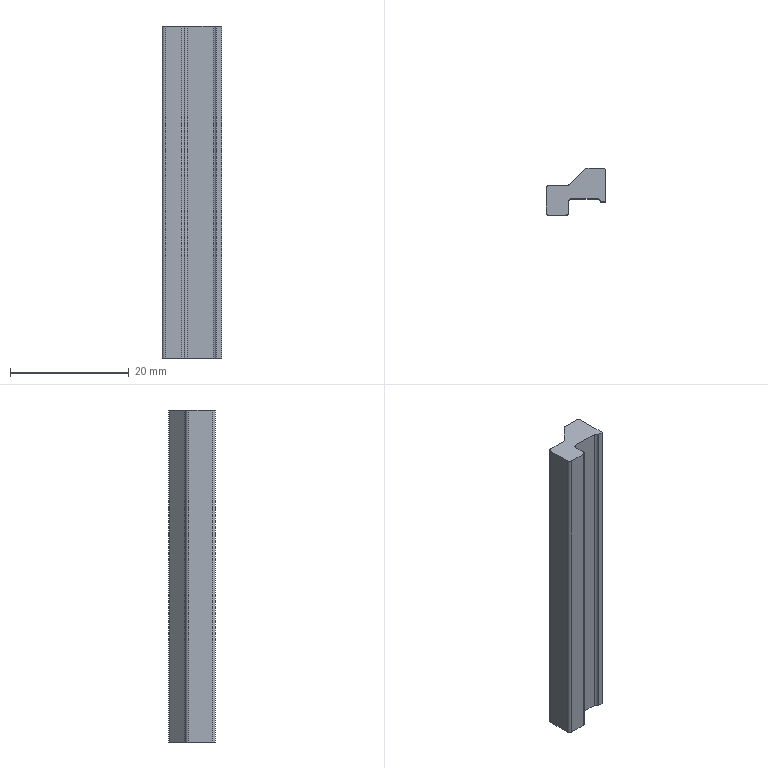Part | NX | features BREP 2 | 2 solids | 40 faces | box 10.056 x 7.899 x 56 mm | volume 5282 mm3 | plane 22 | cylinder 18 | commonest cylinder face diameters 1 x16 188.049 x2
STEP:
#1=CARTESIAN_POINT('',(-0.7746,-1.164,-4.));
#2=VERTEX_POINT('',#1);
#3=CARTESIAN_POINT('',(-0.7746,-1.164,52.));
#4=VERTEX_POINT('',#3);
#5=CARTESIAN_POINT('',(-0.7746,-1.164,0.));
#6=DIRECTION('',(0.,0.,1.));
#7=VECTOR('',#6,1000.);
#8=LINE('',#5,#7);
#9=EDGE_CURVE('',#2,#4,#8,.T.);
#10=ORIENTED_EDGE('',*,*,#9,.T.);
#11=CARTESIAN_POINT('',(-1.275,-1.664,52.));
#12=VERTEX_POINT('',#11);
#13=CARTESIAN_POINT('',(-0.7746,-1.664,52.));
#14=DIRECTION('',(0.,0.,-1.));
#15=DIRECTION('',(1.,0.,0.));
#16=AXIS2_PLACEMENT_3D('',#13,#14,#15);
#17=CIRCLE('',#16,0.5);
#18=EDGE_CURVE('',#12,#4,#17,.T.);
#19=ORIENTED_EDGE('',*,*,#18,.F.);
#20=CARTESIAN_POINT('',(-1.275,-1.664,-4.));
#21=VERTEX_POINT('',#20);
#22=CARTESIAN_POINT('',(-1.275,-1.664,0.));
#23=DIRECTION('',(0.,0.,1.));
#24=VECTOR('',#23,1000.);
#25=LINE('',#22,#24);
#26=EDGE_CURVE('',#21,#12,#25,.T.);
#27=ORIENTED_EDGE('',*,*,#26,.F.);
#28=CARTESIAN_POINT('',(-0.7746,-1.664,-4.));
#29=DIRECTION('',(0.,0.,-1.));
#30=DIRECTION('',(1.,0.,0.));
#31=AXIS2_PLACEMENT_3D('',#28,#29,#30);
#32=CIRCLE('',#31,0.5);
#33=EDGE_CURVE('',#21,#2,#32,.T.);
#34=ORIENTED_EDGE('',*,*,#33,.T.);
#35=EDGE_LOOP('',(#10,#19,#27,#34));
#36=FACE_BOUND('',#35,.T.);
#37=CARTESIAN_POINT('',(-0.7746,-1.664,0.));
#38=DIRECTION('',(0.,0.,1.));
#39=DIRECTION('',(-1.,0.,0.));
#40=AXIS2_PLACEMENT_3D('',#37,#38,#39);
#41=CYLINDRICAL_SURFACE('',#40,0.5);
#42=ADVANCED_FACE('',(#36),#41,.F.);
#43=ORIENTED_EDGE('',*,*,#26,.T.);
#44=CARTESIAN_POINT('',(-1.275,-3.45,52.));
#45=VERTEX_POINT('',#44);
#46=CARTESIAN_POINT('',(-1.275,3.331,52.));
#47=DIRECTION('',(0.,1.,0.));
#48=VECTOR('',#47,1000.);
#49=LINE('',#46,#48);
#50=EDGE_CURVE('',#45,#12,#49,.T.);
#51=ORIENTED_EDGE('',*,*,#50,.F.);
#52=CARTESIAN_POINT('',(-1.275,-3.45,-4.));
#53=VERTEX_POINT('',#52);
#54=CARTESIAN_POINT('',(-1.275,-3.45,0.));
#55=DIRECTION('',(0.,0.,1.));
#56=VECTOR('',#55,1000.);
#57=LINE('',#54,#56);
#58=EDGE_CURVE('',#53,#45,#57,.T.);
#59=ORIENTED_EDGE('',*,*,#58,.F.);
#60=CARTESIAN_POINT('',(-1.275,3.331,-4.));
#61=DIRECTION('',(0.,1.,0.));
#62=VECTOR('',#61,1000.);
#63=LINE('',#60,#62);
#64=EDGE_CURVE('',#53,#21,#63,.T.);
#65=ORIENTED_EDGE('',*,*,#64,.T.);
#66=EDGE_LOOP('',(#43,#51,#59,#65));
#67=FACE_BOUND('',#66,.T.);
#68=CARTESIAN_POINT('',(-1.275,-1.664,0.));
#69=DIRECTION('',(-1.,0.,0.));
#70=DIRECTION('',(0.,1.,0.));
#71=AXIS2_PLACEMENT_3D('',#68,#69,#70);
#72=PLANE('',#71);
#73=ADVANCED_FACE('',(#67),#72,.F.);
#74=ORIENTED_EDGE('',*,*,#58,.T.);
#75=CARTESIAN_POINT('',(-1.775,-3.95,52.));
#76=VERTEX_POINT('',#75);
#77=CARTESIAN_POINT('',(-1.775,-3.45,52.));
#78=DIRECTION('',(0.,0.,1.));
#79=DIRECTION('',(1.,0.,0.));
#80=AXIS2_PLACEMENT_3D('',#77,#78,#79);
#81=CIRCLE('',#80,0.5);
#82=EDGE_CURVE('',#76,#45,#81,.T.);
#83=ORIENTED_EDGE('',*,*,#82,.F.);
#84=CARTESIAN_POINT('',(-1.775,-3.95,-4.));
#85=VERTEX_POINT('',#84);
#86=CARTESIAN_POINT('',(-1.775,-3.95,0.));
#87=DIRECTION('',(0.,0.,1.));
#88=VECTOR('',#87,1000.);
#89=LINE('',#86,#88);
#90=EDGE_CURVE('',#85,#76,#89,.T.);
#91=ORIENTED_EDGE('',*,*,#90,.F.);
#92=CARTESIAN_POINT('',(-1.775,-3.45,-4.));
#93=DIRECTION('',(0.,0.,1.));
#94=DIRECTION('',(1.,0.,0.));
#95=AXIS2_PLACEMENT_3D('',#92,#93,#94);
#96=CIRCLE('',#95,0.5);
#97=EDGE_CURVE('',#85,#53,#96,.T.);
#98=ORIENTED_EDGE('',*,*,#97,.T.);
#99=EDGE_LOOP('',(#74,#83,#91,#98));
#100=FACE_BOUND('',#99,.T.);
#101=CARTESIAN_POINT('',(-1.775,-3.45,0.));
#102=DIRECTION('',(0.,0.,1.));
#103=DIRECTION('',(-1.,0.,0.));
#104=AXIS2_PLACEMENT_3D('',#101,#102,#103);
#105=CYLINDRICAL_SURFACE('',#104,0.5);
#106=ADVANCED_FACE('',(#100),#105,.T.);
#107=ORIENTED_EDGE('',*,*,#90,.T.);
#108=CARTESIAN_POINT('',(-4.531,-3.95,52.));
#109=VERTEX_POINT('',#108);
#110=CARTESIAN_POINT('',(-8.005,-3.95,52.));
#111=DIRECTION('',(1.,0.,0.));
#112=VECTOR('',#111,1000.);
#113=LINE('',#110,#112);
#114=EDGE_CURVE('',#109,#76,#113,.T.);
#115=ORIENTED_EDGE('',*,*,#114,.F.);
#116=CARTESIAN_POINT('',(-4.531,-3.95,-4.));
#117=VERTEX_POINT('',#116);
#118=CARTESIAN_POINT('',(-4.531,-3.95,0.));
#119=DIRECTION('',(0.,0.,1.));
#120=VECTOR('',#119,1000.);
#121=LINE('',#118,#120);
#122=EDGE_CURVE('',#117,#109,#121,.T.);
#123=ORIENTED_EDGE('',*,*,#122,.F.);
#124=CARTESIAN_POINT('',(-8.005,-3.95,-4.));
#125=DIRECTION('',(1.,0.,0.));
#126=VECTOR('',#125,1000.);
#127=LINE('',#124,#126);
#128=EDGE_CURVE('',#117,#85,#127,.T.);
#129=ORIENTED_EDGE('',*,*,#128,.T.);
#130=EDGE_LOOP('',(#107,#115,#123,#129));
#131=FACE_BOUND('',#130,.T.);
#132=CARTESIAN_POINT('',(-1.775,-3.95,0.));
#133=DIRECTION('',(0.,1.,0.));
#134=DIRECTION('',(1.,0.,0.));
#135=AXIS2_PLACEMENT_3D('',#132,#133,#134);
#136=PLANE('',#135);
#137=ADVANCED_FACE('',(#131),#136,.F.);
#138=ORIENTED_EDGE('',*,*,#122,.T.);
#139=CARTESIAN_POINT('',(-5.031,-3.45,52.));
#140=VERTEX_POINT('',#139);
#141=CARTESIAN_POINT('',(-4.531,-3.45,52.));
#142=DIRECTION('',(0.,0.,1.));
#143=DIRECTION('',(1.,0.,0.));
#144=AXIS2_PLACEMENT_3D('',#141,#142,#143);
#145=CIRCLE('',#144,0.5);
#146=EDGE_CURVE('',#140,#109,#145,.T.);
#147=ORIENTED_EDGE('',*,*,#146,.F.);
#148=CARTESIAN_POINT('',(-5.031,-3.45,-4.));
#149=VERTEX_POINT('',#148);
#150=CARTESIAN_POINT('',(-5.031,-3.45,0.));
#151=DIRECTION('',(0.,0.,1.));
#152=VECTOR('',#151,1000.);
#153=LINE('',#150,#152);
#154=EDGE_CURVE('',#149,#140,#153,.T.);
#155=ORIENTED_EDGE('',*,*,#154,.F.);
#156=CARTESIAN_POINT('',(-4.531,-3.45,-4.));
#157=DIRECTION('',(0.,0.,1.));
#158=DIRECTION('',(1.,0.,0.));
#159=AXIS2_PLACEMENT_3D('',#156,#157,#158);
#160=CIRCLE('',#159,0.5);
#161=EDGE_CURVE('',#149,#117,#160,.T.);
#162=ORIENTED_EDGE('',*,*,#161,.T.);
#163=EDGE_LOOP('',(#138,#147,#155,#162));
#164=FACE_BOUND('',#163,.T.);
#165=CARTESIAN_POINT('',(-4.531,-3.45,0.));
#166=DIRECTION('',(0.,0.,1.));
#167=DIRECTION('',(-1.,0.,0.));
#168=AXIS2_PLACEMENT_3D('',#165,#166,#167);
#169=CYLINDRICAL_SURFACE('',#168,0.5);
#170=ADVANCED_FACE('',(#164),#169,.T.);
#171=ORIENTED_EDGE('',*,*,#154,.T.);
#172=CARTESIAN_POINT('',(-5.031,0.5504,52.));
#173=VERTEX_POINT('',#172);
#174=CARTESIAN_POINT('',(-5.031,3.331,52.));
#175=DIRECTION('',(0.,-1.,0.));
#176=VECTOR('',#175,1000.);
#177=LINE('',#174,#176);
#178=EDGE_CURVE('',#173,#140,#177,.T.);
#179=ORIENTED_EDGE('',*,*,#178,.F.);
#180=CARTESIAN_POINT('',(-5.031,0.5504,-4.));
#181=VERTEX_POINT('',#180);
#182=CARTESIAN_POINT('',(-5.031,0.5504,0.));
#183=DIRECTION('',(0.,0.,1.));
#184=VECTOR('',#183,1000.);
#185=LINE('',#182,#184);
#186=EDGE_CURVE('',#181,#173,#185,.T.);
#187=ORIENTED_EDGE('',*,*,#186,.F.);
#188=CARTESIAN_POINT('',(-5.031,3.331,-4.));
#189=DIRECTION('',(0.,-1.,0.));
#190=VECTOR('',#189,1000.);
#191=LINE('',#188,#190);
#192=EDGE_CURVE('',#181,#149,#191,.T.);
#193=ORIENTED_EDGE('',*,*,#192,.T.);
#194=EDGE_LOOP('',(#171,#179,#187,#193));
#195=FACE_BOUND('',#194,.T.);
#196=CARTESIAN_POINT('',(-5.031,-3.45,0.));
#197=DIRECTION('',(1.,0.,0.));
#198=DIRECTION('',(0.,-1.,0.));
#199=AXIS2_PLACEMENT_3D('',#196,#197,#198);
#200=PLANE('',#199);
#201=ADVANCED_FACE('',(#195),#200,.F.);
#202=ORIENTED_EDGE('',*,*,#186,.T.);
#203=CARTESIAN_POINT('',(-4.531,1.05,52.));
#204=VERTEX_POINT('',#203);
#205=CARTESIAN_POINT('',(-4.531,0.5504,52.));
#206=DIRECTION('',(0.,0.,1.));
#207=DIRECTION('',(1.,0.,0.));
#208=AXIS2_PLACEMENT_3D('',#205,#206,#207);
#209=CIRCLE('',#208,0.5);
#210=EDGE_CURVE('',#204,#173,#209,.T.);
#211=ORIENTED_EDGE('',*,*,#210,.F.);
#212=CARTESIAN_POINT('',(-4.531,1.05,-4.));
#213=VERTEX_POINT('',#212);
#214=CARTESIAN_POINT('',(-4.531,1.05,0.));
#215=DIRECTION('',(0.,0.,1.));
#216=VECTOR('',#215,1000.);
#217=LINE('',#214,#216);
#218=EDGE_CURVE('',#213,#204,#217,.T.);
#219=ORIENTED_EDGE('',*,*,#218,.F.);
#220=CARTESIAN_POINT('',(-4.531,0.5504,-4.));
#221=DIRECTION('',(0.,0.,1.));
#222=DIRECTION('',(1.,0.,0.));
#223=AXIS2_PLACEMENT_3D('',#220,#221,#222);
#224=CIRCLE('',#223,0.5);
#225=EDGE_CURVE('',#213,#181,#224,.T.);
#226=ORIENTED_EDGE('',*,*,#225,.T.);
#227=EDGE_LOOP('',(#202,#211,#219,#226));
#228=FACE_BOUND('',#227,.T.);
#229=CARTESIAN_POINT('',(-4.531,0.5504,0.));
#230=DIRECTION('',(0.,0.,1.));
#231=DIRECTION('',(-1.,0.,0.));
#232=AXIS2_PLACEMENT_3D('',#229,#230,#231);
#233=CYLINDRICAL_SURFACE('',#232,0.5);
#234=ADVANCED_FACE('',(#228),#233,.T.);
#235=ORIENTED_EDGE('',*,*,#218,.T.);
#236=CARTESIAN_POINT('',(-1.482,1.05,52.));
#237=VERTEX_POINT('',#236);
#238=CARTESIAN_POINT('',(-8.005,1.05,52.));
#239=DIRECTION('',(-1.,0.,0.));
#240=VECTOR('',#239,1000.);
#241=LINE('',#238,#240);
#242=EDGE_CURVE('',#237,#204,#241,.T.);
#243=ORIENTED_EDGE('',*,*,#242,.F.);
#244=CARTESIAN_POINT('',(-1.482,1.05,-4.));
#245=VERTEX_POINT('',#244);
#246=CARTESIAN_POINT('',(-1.482,1.05,0.));
#247=DIRECTION('',(0.,0.,1.));
#248=VECTOR('',#247,1000.);
#249=LINE('',#246,#248);
#250=EDGE_CURVE('',#245,#237,#249,.T.);
#251=ORIENTED_EDGE('',*,*,#250,.F.);
#252=CARTESIAN_POINT('',(-8.005,1.05,-4.));
#253=DIRECTION('',(-1.,0.,0.));
#254=VECTOR('',#253,1000.);
#255=LINE('',#252,#254);
#256=EDGE_CURVE('',#245,#213,#255,.T.);
#257=ORIENTED_EDGE('',*,*,#256,.T.);
#258=EDGE_LOOP('',(#235,#243,#251,#257));
#259=FACE_BOUND('',#258,.T.);
#260=CARTESIAN_POINT('',(-4.531,1.05,0.));
#261=DIRECTION('',(0.,-1.,0.));
#262=DIRECTION('',(-1.,0.,0.));
#263=AXIS2_PLACEMENT_3D('',#260,#261,#262);
#264=PLANE('',#263);
#265=ADVANCED_FACE('',(#259),#264,.F.);
#266=ORIENTED_EDGE('',*,*,#250,.T.);
#267=CARTESIAN_POINT('',(-1.128,1.197,52.));
#268=VERTEX_POINT('',#267);
#269=CARTESIAN_POINT('',(-1.482,1.55,52.));
#270=DIRECTION('',(0.,0.,-1.));
#271=DIRECTION('',(1.,0.,0.));
#272=AXIS2_PLACEMENT_3D('',#269,#270,#271);
#273=CIRCLE('',#272,0.5);
#274=EDGE_CURVE('',#268,#237,#273,.T.);
#275=ORIENTED_EDGE('',*,*,#274,.F.);
#276=CARTESIAN_POINT('',(-1.128,1.197,-4.));
#277=VERTEX_POINT('',#276);
#278=CARTESIAN_POINT('',(-1.128,1.197,0.));
#279=DIRECTION('',(0.,0.,1.));
#280=VECTOR('',#279,1000.);
#281=LINE('',#278,#280);
#282=EDGE_CURVE('',#277,#268,#281,.T.);
#283=ORIENTED_EDGE('',*,*,#282,.F.);
#284=CARTESIAN_POINT('',(-1.482,1.55,-4.));
#285=DIRECTION('',(0.,0.,-1.));
#286=DIRECTION('',(1.,0.,0.));
#287=AXIS2_PLACEMENT_3D('',#284,#285,#286);
#288=CIRCLE('',#287,0.5);
#289=EDGE_CURVE('',#277,#245,#288,.T.);
#290=ORIENTED_EDGE('',*,*,#289,.T.);
#291=EDGE_LOOP('',(#266,#275,#283,#290));
#292=FACE_BOUND('',#291,.T.);
#293=CARTESIAN_POINT('',(-1.482,1.55,0.));
#294=DIRECTION('',(0.,0.,1.));
#295=DIRECTION('',(-1.,0.,0.));
#296=AXIS2_PLACEMENT_3D('',#293,#294,#295);
#297=CYLINDRICAL_SURFACE('',#296,0.5);
#298=ADVANCED_FACE('',(#292),#297,.F.);
#299=ORIENTED_EDGE('',*,*,#282,.T.);
#300=CARTESIAN_POINT('',(1.478,3.803,52.));
#301=VERTEX_POINT('',#300);
#302=CARTESIAN_POINT('',(-1.128,1.197,52.));
#303=DIRECTION('',(-0.7071,-0.7071,0.));
#304=VECTOR('',#303,1000.);
#305=LINE('',#302,#304);
#306=EDGE_CURVE('',#301,#268,#305,.T.);
#307=ORIENTED_EDGE('',*,*,#306,.F.);
#308=CARTESIAN_POINT('',(1.478,3.803,-4.));
#309=VERTEX_POINT('',#308);
#310=CARTESIAN_POINT('',(1.478,3.803,0.));
#311=DIRECTION('',(0.,0.,1.));
#312=VECTOR('',#311,1000.);
#313=LINE('',#310,#312);
#314=EDGE_CURVE('',#309,#301,#313,.T.);
#315=ORIENTED_EDGE('',*,*,#314,.F.);
#316=CARTESIAN_POINT('',(-1.128,1.197,-4.));
#317=DIRECTION('',(-0.7071,-0.7071,0.));
#318=VECTOR('',#317,1000.);
#319=LINE('',#316,#318);
#320=EDGE_CURVE('',#309,#277,#319,.T.);
#321=ORIENTED_EDGE('',*,*,#320,.T.);
#322=EDGE_LOOP('',(#299,#307,#315,#321));
#323=FACE_BOUND('',#322,.T.);
#324=CARTESIAN_POINT('',(-1.128,1.197,0.));
#325=DIRECTION('',(0.7071,-0.7071,0.));
#326=DIRECTION('',(-0.7071,-0.7071,0.));
#327=AXIS2_PLACEMENT_3D('',#324,#325,#326);
#328=PLANE('',#327);
#329=ADVANCED_FACE('',(#323),#328,.F.);
#330=ORIENTED_EDGE('',*,*,#314,.T.);
#331=CARTESIAN_POINT('',(1.832,3.95,52.));
#332=VERTEX_POINT('',#331);
#333=CARTESIAN_POINT('',(1.832,3.45,52.));
#334=DIRECTION('',(0.,0.,1.));
#335=DIRECTION('',(1.,0.,0.));
#336=AXIS2_PLACEMENT_3D('',#333,#334,#335);
#337=CIRCLE('',#336,0.5);
#338=EDGE_CURVE('',#332,#301,#337,.T.);
#339=ORIENTED_EDGE('',*,*,#338,.F.);
#340=CARTESIAN_POINT('',(1.832,3.95,-4.));
#341=VERTEX_POINT('',#340);
#342=CARTESIAN_POINT('',(1.832,3.95,0.));
#343=DIRECTION('',(0.,0.,1.));
#344=VECTOR('',#343,1000.);
#345=LINE('',#342,#344);
#346=EDGE_CURVE('',#341,#332,#345,.T.);
#347=ORIENTED_EDGE('',*,*,#346,.F.);
#348=CARTESIAN_POINT('',(1.832,3.45,-4.));
#349=DIRECTION('',(0.,0.,1.));
#350=DIRECTION('',(1.,0.,0.));
#351=AXIS2_PLACEMENT_3D('',#348,#349,#350);
#352=CIRCLE('',#351,0.5);
#353=EDGE_CURVE('',#341,#309,#352,.T.);
#354=ORIENTED_EDGE('',*,*,#353,.T.);
#355=EDGE_LOOP('',(#330,#339,#347,#354));
#356=FACE_BOUND('',#355,.T.);
#357=CARTESIAN_POINT('',(1.832,3.45,0.));
#358=DIRECTION('',(0.,0.,1.));
#359=DIRECTION('',(-1.,0.,0.));
#360=AXIS2_PLACEMENT_3D('',#357,#358,#359);
#361=CYLINDRICAL_SURFACE('',#360,0.5);
#362=ADVANCED_FACE('',(#356),#361,.T.);
#363=ORIENTED_EDGE('',*,*,#346,.T.);
#364=CARTESIAN_POINT('',(4.525,3.95,52.));
#365=VERTEX_POINT('',#364);
#366=CARTESIAN_POINT('',(-8.005,3.95,52.));
#367=DIRECTION('',(-1.,0.,0.));
#368=VECTOR('',#367,1000.);
#369=LINE('',#366,#368);
#370=EDGE_CURVE('',#365,#332,#369,.T.);
#371=ORIENTED_EDGE('',*,*,#370,.F.);
#372=CARTESIAN_POINT('',(4.525,3.95,-4.));
#373=VERTEX_POINT('',#372);
#374=CARTESIAN_POINT('',(4.525,3.95,0.));
#375=DIRECTION('',(0.,0.,1.));
#376=VECTOR('',#375,1000.);
#377=LINE('',#374,#376);
#378=EDGE_CURVE('',#373,#365,#377,.T.);
#379=ORIENTED_EDGE('',*,*,#378,.F.);
#380=CARTESIAN_POINT('',(-8.005,3.95,-4.));
#381=DIRECTION('',(-1.,0.,0.));
#382=VECTOR('',#381,1000.);
#383=LINE('',#380,#382);
#384=EDGE_CURVE('',#373,#341,#383,.T.);
#385=ORIENTED_EDGE('',*,*,#384,.T.);
#386=EDGE_LOOP('',(#363,#371,#379,#385));
#387=FACE_BOUND('',#386,.T.);
#388=CARTESIAN_POINT('',(1.832,3.95,0.));
#389=DIRECTION('',(0.,-1.,0.));
#390=DIRECTION('',(-1.,0.,0.));
#391=AXIS2_PLACEMENT_3D('',#388,#389,#390);
#392=PLANE('',#391);
#393=ADVANCED_FACE('',(#387),#392,.F.);
#394=ORIENTED_EDGE('',*,*,#378,.T.);
#395=CARTESIAN_POINT('',(5.025,3.45,52.));
#396=VERTEX_POINT('',#395);
#397=CARTESIAN_POINT('',(4.525,3.45,52.));
#398=DIRECTION('',(0.,0.,1.));
#399=DIRECTION('',(1.,0.,0.));
#400=AXIS2_PLACEMENT_3D('',#397,#398,#399);
#401=CIRCLE('',#400,0.5);
#402=EDGE_CURVE('',#396,#365,#401,.T.);
#403=ORIENTED_EDGE('',*,*,#402,.F.);
#404=CARTESIAN_POINT('',(5.025,3.45,-4.));
#405=VERTEX_POINT('',#404);
#406=CARTESIAN_POINT('',(5.025,3.45,0.));
#407=DIRECTION('',(0.,0.,1.));
#408=VECTOR('',#407,1000.);
#409=LINE('',#406,#408);
#410=EDGE_CURVE('',#405,#396,#409,.T.);
#411=ORIENTED_EDGE('',*,*,#410,.F.);
#412=CARTESIAN_POINT('',(4.525,3.45,-4.));
#413=DIRECTION('',(0.,0.,1.));
#414=DIRECTION('',(1.,0.,0.));
#415=AXIS2_PLACEMENT_3D('',#412,#413,#414);
#416=CIRCLE('',#415,0.5);
#417=EDGE_CURVE('',#405,#373,#416,.T.);
#418=ORIENTED_EDGE('',*,*,#417,.T.);
#419=EDGE_LOOP('',(#394,#403,#411,#418));
#420=FACE_BOUND('',#419,.T.);
#421=CARTESIAN_POINT('',(4.525,3.45,0.));
#422=DIRECTION('',(0.,0.,1.));
#423=DIRECTION('',(-1.,0.,0.));
#424=AXIS2_PLACEMENT_3D('',#421,#422,#423);
#425=CYLINDRICAL_SURFACE('',#424,0.5);
#426=ADVANCED_FACE('',(#420),#425,.T.);
#427=ORIENTED_EDGE('',*,*,#410,.T.);
#428=CARTESIAN_POINT('',(5.025,-1.169,52.));
#429=VERTEX_POINT('',#428);
#430=CARTESIAN_POINT('',(5.025,3.331,52.));
#431=DIRECTION('',(0.,1.,0.));
#432=VECTOR('',#431,1000.);
#433=LINE('',#430,#432);
#434=EDGE_CURVE('',#429,#396,#433,.T.);
#435=ORIENTED_EDGE('',*,*,#434,.F.);
#436=CARTESIAN_POINT('',(5.025,-1.169,-4.));
#437=VERTEX_POINT('',#436);
#438=CARTESIAN_POINT('',(5.025,-1.169,52.));
#439=CARTESIAN_POINT('',(5.025,-1.169,33.333));
#440=CARTESIAN_POINT('',(5.025,-1.169,14.667));
#441=CARTESIAN_POINT('',(5.025,-1.169,-4.));
#442=B_SPLINE_CURVE_WITH_KNOTS('',3,(#438,#439,#440,#441),.UNSPECIFIED.,.F.,.F.,(4,4),(0.,1.),.UNSPECIFIED.);
#443=EDGE_CURVE('',#437,#429,#442,.F.);
#444=ORIENTED_EDGE('',*,*,#443,.F.);
#445=CARTESIAN_POINT('',(5.025,3.331,-4.));
#446=DIRECTION('',(0.,1.,0.));
#447=VECTOR('',#446,1000.);
#448=LINE('',#445,#447);
#449=EDGE_CURVE('',#437,#405,#448,.T.);
#450=ORIENTED_EDGE('',*,*,#449,.T.);
#451=EDGE_LOOP('',(#427,#435,#444,#450));
#452=FACE_BOUND('',#451,.T.);
#453=CARTESIAN_POINT('',(5.025,3.45,0.));
#454=DIRECTION('',(-1.,0.,0.));
#455=DIRECTION('',(0.,1.,0.));
#456=AXIS2_PLACEMENT_3D('',#453,#454,#455);
#457=PLANE('',#456);
#458=ADVANCED_FACE('',(#452),#457,.F.);
#459=ORIENTED_EDGE('',*,*,#443,.T.);
#460=CARTESIAN_POINT('',(5.01,-1.685,52.));
#461=VERTEX_POINT('',#460);
#462=CARTESIAN_POINT('',(-88.969,1.235,52.));
#463=DIRECTION('',(0.,0.,1.));
#464=DIRECTION('',(1.,0.,0.));
#465=AXIS2_PLACEMENT_3D('',#462,#463,#464);
#466=CIRCLE('',#465,94.024);
#467=EDGE_CURVE('',#461,#429,#466,.T.);
#468=ORIENTED_EDGE('',*,*,#467,.F.);
#469=CARTESIAN_POINT('',(5.01,-1.685,-4.));
#470=VERTEX_POINT('',#469);
#471=CARTESIAN_POINT('',(5.01,-1.685,0.));
#472=DIRECTION('',(0.,0.,1.));
#473=VECTOR('',#472,1000.);
#474=LINE('',#471,#473);
#475=EDGE_CURVE('',#470,#461,#474,.T.);
#476=ORIENTED_EDGE('',*,*,#475,.F.);
#477=CARTESIAN_POINT('',(-88.969,1.235,-4.));
#478=DIRECTION('',(0.,0.,1.));
#479=DIRECTION('',(1.,0.,0.));
#480=AXIS2_PLACEMENT_3D('',#477,#478,#479);
#481=CIRCLE('',#480,94.024);
#482=EDGE_CURVE('',#470,#437,#481,.T.);
#483=ORIENTED_EDGE('',*,*,#482,.T.);
#484=EDGE_LOOP('',(#459,#468,#476,#483));
#485=FACE_BOUND('',#484,.T.);
#486=CARTESIAN_POINT('',(-88.969,1.235,0.));
#487=DIRECTION('',(0.,0.,1.));
#488=DIRECTION('',(-1.,0.,0.));
#489=AXIS2_PLACEMENT_3D('',#486,#487,#488);
#490=CYLINDRICAL_SURFACE('',#489,94.024);
#491=ADVANCED_FACE('',(#485),#490,.T.);
#492=ORIENTED_EDGE('',*,*,#475,.T.);
#493=CARTESIAN_POINT('',(4.105,-1.685,52.));
#494=VERTEX_POINT('',#493);
#495=CARTESIAN_POINT('',(-8.005,-1.685,52.));
#496=DIRECTION('',(1.,0.,0.));
#497=VECTOR('',#496,1000.);
#498=LINE('',#495,#497);
#499=EDGE_CURVE('',#494,#461,#498,.T.);
#500=ORIENTED_EDGE('',*,*,#499,.F.);
#501=CARTESIAN_POINT('',(4.105,-1.685,-4.));
#502=VERTEX_POINT('',#501);
#503=CARTESIAN_POINT('',(4.105,-1.685,0.));
#504=DIRECTION('',(0.,0.,1.));
#505=VECTOR('',#504,1000.);
#506=LINE('',#503,#505);
#507=EDGE_CURVE('',#502,#494,#506,.T.);
#508=ORIENTED_EDGE('',*,*,#507,.F.);
#509=CARTESIAN_POINT('',(-8.005,-1.685,-4.));
#510=DIRECTION('',(1.,0.,0.));
#511=VECTOR('',#510,1000.);
#512=LINE('',#509,#511);
#513=EDGE_CURVE('',#502,#470,#512,.T.);
#514=ORIENTED_EDGE('',*,*,#513,.T.);
#515=EDGE_LOOP('',(#492,#500,#508,#514));
#516=FACE_BOUND('',#515,.T.);
#517=CARTESIAN_POINT('',(-8.005,-1.685,0.));
#518=DIRECTION('',(0.,-1.,0.));
#519=DIRECTION('',(-1.,0.,0.));
#520=AXIS2_PLACEMENT_3D('',#517,#518,#519);
#521=PLANE('',#520);
#522=ADVANCED_FACE('',(#516),#521,.T.);
#523=ORIENTED_EDGE('',*,*,#507,.T.);
#524=CARTESIAN_POINT('',(3.605,-1.164,52.));
#525=VERTEX_POINT('',#524);
#526=CARTESIAN_POINT('',(3.605,-1.664,52.));
#527=DIRECTION('',(0.,0.,-1.));
#528=DIRECTION('',(1.,0.,0.));
#529=AXIS2_PLACEMENT_3D('',#526,#527,#528);
#530=CIRCLE('',#529,0.5);
#531=EDGE_CURVE('',#525,#494,#530,.T.);
#532=ORIENTED_EDGE('',*,*,#531,.F.);
#533=CARTESIAN_POINT('',(3.605,-1.164,-4.));
#534=VERTEX_POINT('',#533);
#535=CARTESIAN_POINT('',(3.605,-1.164,0.));
#536=DIRECTION('',(0.,0.,1.));
#537=VECTOR('',#536,1000.);
#538=LINE('',#535,#537);
#539=EDGE_CURVE('',#534,#525,#538,.T.);
#540=ORIENTED_EDGE('',*,*,#539,.F.);
#541=CARTESIAN_POINT('',(3.605,-1.664,-4.));
#542=DIRECTION('',(0.,0.,-1.));
#543=DIRECTION('',(1.,0.,0.));
#544=AXIS2_PLACEMENT_3D('',#541,#542,#543);
#545=CIRCLE('',#544,0.5);
#546=EDGE_CURVE('',#534,#502,#545,.T.);
#547=ORIENTED_EDGE('',*,*,#546,.T.);
#548=EDGE_LOOP('',(#523,#532,#540,#547));
#549=FACE_BOUND('',#548,.T.);
#550=CARTESIAN_POINT('',(3.605,-1.664,0.));
#551=DIRECTION('',(0.,0.,1.));
#552=DIRECTION('',(-1.,0.,0.));
#553=AXIS2_PLACEMENT_3D('',#550,#551,#552);
#554=CYLINDRICAL_SURFACE('',#553,0.5);
#555=ADVANCED_FACE('',(#549),#554,.F.);
#556=CARTESIAN_POINT('',(-8.005,-1.164,-4.));
#557=DIRECTION('',(1.,0.,0.));
#558=VECTOR('',#557,1000.);
#559=LINE('',#556,#558);
#560=EDGE_CURVE('',#2,#534,#559,.T.);
#561=ORIENTED_EDGE('',*,*,#560,.T.);
#562=ORIENTED_EDGE('',*,*,#539,.T.);
#563=CARTESIAN_POINT('',(-8.005,-1.164,52.));
#564=DIRECTION('',(1.,0.,0.));
#565=VECTOR('',#564,1000.);
#566=LINE('',#563,#565);
#567=EDGE_CURVE('',#4,#525,#566,.T.);
#568=ORIENTED_EDGE('',*,*,#567,.F.);
#569=ORIENTED_EDGE('',*,*,#9,.F.);
#570=EDGE_LOOP('',(#561,#562,#568,#569));
#571=FACE_BOUND('',#570,.T.);
#572=CARTESIAN_POINT('',(3.605,-1.164,0.));
#573=DIRECTION('',(0.,1.,0.));
#574=DIRECTION('',(1.,0.,0.));
#575=AXIS2_PLACEMENT_3D('',#572,#573,#574);
#576=PLANE('',#575);
#577=ADVANCED_FACE('',(#571),#576,.F.);
#578=ORIENTED_EDGE('',*,*,#531,.T.);
#579=ORIENTED_EDGE('',*,*,#499,.T.);
#580=ORIENTED_EDGE('',*,*,#467,.T.);
#581=ORIENTED_EDGE('',*,*,#434,.T.);
#582=ORIENTED_EDGE('',*,*,#402,.T.);
#583=ORIENTED_EDGE('',*,*,#370,.T.);
#584=ORIENTED_EDGE('',*,*,#338,.T.);
#585=ORIENTED_EDGE('',*,*,#306,.T.);
#586=ORIENTED_EDGE('',*,*,#274,.T.);
#587=ORIENTED_EDGE('',*,*,#242,.T.);
#588=ORIENTED_EDGE('',*,*,#210,.T.);
#589=ORIENTED_EDGE('',*,*,#178,.T.);
#590=ORIENTED_EDGE('',*,*,#146,.T.);
#591=ORIENTED_EDGE('',*,*,#114,.T.);
#592=ORIENTED_EDGE('',*,*,#82,.T.);
#593=ORIENTED_EDGE('',*,*,#50,.T.);
#594=ORIENTED_EDGE('',*,*,#18,.T.);
#595=ORIENTED_EDGE('',*,*,#567,.T.);
#596=EDGE_LOOP('',(#578,#579,#580,#581,#582,#583,#584,#585,#586,#587,#588,#589,#590,#591,#592,#593,#594,#595));
#597=FACE_BOUND('',#596,.T.);
#598=CARTESIAN_POINT('',(-8.005,3.331,52.));
#599=DIRECTION('',(0.,0.,1.));
#600=DIRECTION('',(-1.,0.,0.));
#601=AXIS2_PLACEMENT_3D('',#598,#599,#600);
#602=PLANE('',#601);
#603=ADVANCED_FACE('',(#597),#602,.T.);
#604=ORIENTED_EDGE('',*,*,#546,.F.);
#605=ORIENTED_EDGE('',*,*,#560,.F.);
#606=ORIENTED_EDGE('',*,*,#33,.F.);
#607=ORIENTED_EDGE('',*,*,#64,.F.);
#608=ORIENTED_EDGE('',*,*,#97,.F.);
#609=ORIENTED_EDGE('',*,*,#128,.F.);
#610=ORIENTED_EDGE('',*,*,#161,.F.);
#611=ORIENTED_EDGE('',*,*,#192,.F.);
#612=ORIENTED_EDGE('',*,*,#225,.F.);
#613=ORIENTED_EDGE('',*,*,#256,.F.);
#614=ORIENTED_EDGE('',*,*,#289,.F.);
#615=ORIENTED_EDGE('',*,*,#320,.F.);
#616=ORIENTED_EDGE('',*,*,#353,.F.);
#617=ORIENTED_EDGE('',*,*,#384,.F.);
#618=ORIENTED_EDGE('',*,*,#417,.F.);
#619=ORIENTED_EDGE('',*,*,#449,.F.);
#620=ORIENTED_EDGE('',*,*,#482,.F.);
#621=ORIENTED_EDGE('',*,*,#513,.F.);
#622=EDGE_LOOP('',(#604,#605,#606,#607,#608,#609,#610,#611,#612,#613,#614,#615,#616,#617,#618,#619,#620,#621));
#623=FACE_BOUND('',#622,.T.);
#624=CARTESIAN_POINT('',(-8.005,3.331,-4.));
#625=DIRECTION('',(0.,0.,1.));
#626=DIRECTION('',(-1.,0.,0.));
#627=AXIS2_PLACEMENT_3D('',#624,#625,#626);
#628=PLANE('',#627);
#629=ADVANCED_FACE('',(#623),#628,.F.);
#630=CLOSED_SHELL('',(#42,#73,#106,#137,#170,#201,#234,#265,#298,#329,#362,#393,#426,#458,#491,#522,#555,#577,#603,#629));
#631=MANIFOLD_SOLID_BREP('',#630);
#632=CARTESIAN_POINT('',(-0.7746,-1.164,-4.));
#633=VERTEX_POINT('',#632);
#634=CARTESIAN_POINT('',(-0.7746,-1.164,52.));
#635=VERTEX_POINT('',#634);
#636=CARTESIAN_POINT('',(-0.7746,-1.164,0.));
#637=DIRECTION('',(0.,0.,1.));
#638=VECTOR('',#637,1000.);
#639=LINE('',#636,#638);
#640=EDGE_CURVE('',#633,#635,#639,.T.);
#641=ORIENTED_EDGE('',*,*,#640,.T.);
#642=CARTESIAN_POINT('',(-1.275,-1.664,52.));
#643=VERTEX_POINT('',#642);
#644=CARTESIAN_POINT('',(-0.7746,-1.664,52.));
#645=DIRECTION('',(0.,0.,-1.));
#646=DIRECTION('',(1.,0.,0.));
#647=AXIS2_PLACEMENT_3D('',#644,#645,#646);
#648=CIRCLE('',#647,0.5);
#649=EDGE_CURVE('',#643,#635,#648,.T.);
#650=ORIENTED_EDGE('',*,*,#649,.F.);
#651=CARTESIAN_POINT('',(-1.275,-1.664,-4.));
#652=VERTEX_POINT('',#651);
#653=CARTESIAN_POINT('',(-1.275,-1.664,0.));
#654=DIRECTION('',(0.,0.,1.));
#655=VECTOR('',#654,1000.);
#656=LINE('',#653,#655);
#657=EDGE_CURVE('',#652,#643,#656,.T.);
#658=ORIENTED_EDGE('',*,*,#657,.F.);
#659=CARTESIAN_POINT('',(-0.7746,-1.664,-4.));
#660=DIRECTION('',(0.,0.,-1.));
#661=DIRECTION('',(1.,0.,0.));
#662=AXIS2_PLACEMENT_3D('',#659,#660,#661);
#663=CIRCLE('',#662,0.5);
#664=EDGE_CURVE('',#652,#633,#663,.T.);
#665=ORIENTED_EDGE('',*,*,#664,.T.);
#666=EDGE_LOOP('',(#641,#650,#658,#665));
#667=FACE_BOUND('',#666,.T.);
#668=CARTESIAN_POINT('',(-0.7746,-1.664,0.));
#669=DIRECTION('',(0.,0.,1.));
#670=DIRECTION('',(-1.,0.,0.));
#671=AXIS2_PLACEMENT_3D('',#668,#669,#670);
#672=CYLINDRICAL_SURFACE('',#671,0.5);
#673=ADVANCED_FACE('',(#667),#672,.F.);
#674=ORIENTED_EDGE('',*,*,#657,.T.);
#675=CARTESIAN_POINT('',(-1.275,-3.45,52.));
#676=VERTEX_POINT('',#675);
#677=CARTESIAN_POINT('',(-1.275,3.331,52.));
#678=DIRECTION('',(0.,1.,0.));
#679=VECTOR('',#678,1000.);
#680=LINE('',#677,#679);
#681=EDGE_CURVE('',#676,#643,#680,.T.);
#682=ORIENTED_EDGE('',*,*,#681,.F.);
#683=CARTESIAN_POINT('',(-1.275,-3.45,-4.));
#684=VERTEX_POINT('',#683);
#685=CARTESIAN_POINT('',(-1.275,-3.45,0.));
#686=DIRECTION('',(0.,0.,1.));
#687=VECTOR('',#686,1000.);
#688=LINE('',#685,#687);
#689=EDGE_CURVE('',#684,#676,#688,.T.);
#690=ORIENTED_EDGE('',*,*,#689,.F.);
#691=CARTESIAN_POINT('',(-1.275,3.331,-4.));
#692=DIRECTION('',(0.,1.,0.));
#693=VECTOR('',#692,1000.);
#694=LINE('',#691,#693);
#695=EDGE_CURVE('',#684,#652,#694,.T.);
#696=ORIENTED_EDGE('',*,*,#695,.T.);
#697=EDGE_LOOP('',(#674,#682,#690,#696));
#698=FACE_BOUND('',#697,.T.);
#699=CARTESIAN_POINT('',(-1.275,-1.664,0.));
#700=DIRECTION('',(-1.,0.,0.));
#701=DIRECTION('',(0.,1.,0.));
#702=AXIS2_PLACEMENT_3D('',#699,#700,#701);
#703=PLANE('',#702);
#704=ADVANCED_FACE('',(#698),#703,.F.);
#705=ORIENTED_EDGE('',*,*,#689,.T.);
#706=CARTESIAN_POINT('',(-1.775,-3.95,52.));
#707=VERTEX_POINT('',#706);
#708=CARTESIAN_POINT('',(-1.775,-3.45,52.));
#709=DIRECTION('',(0.,0.,1.));
#710=DIRECTION('',(1.,0.,0.));
#711=AXIS2_PLACEMENT_3D('',#708,#709,#710);
#712=CIRCLE('',#711,0.5);
#713=EDGE_CURVE('',#707,#676,#712,.T.);
#714=ORIENTED_EDGE('',*,*,#713,.F.);
#715=CARTESIAN_POINT('',(-1.775,-3.95,-4.));
#716=VERTEX_POINT('',#715);
#717=CARTESIAN_POINT('',(-1.775,-3.95,0.));
#718=DIRECTION('',(0.,0.,1.));
#719=VECTOR('',#718,1000.);
#720=LINE('',#717,#719);
#721=EDGE_CURVE('',#716,#707,#720,.T.);
#722=ORIENTED_EDGE('',*,*,#721,.F.);
#723=CARTESIAN_POINT('',(-1.775,-3.45,-4.));
#724=DIRECTION('',(0.,0.,1.));
#725=DIRECTION('',(1.,0.,0.));
#726=AXIS2_PLACEMENT_3D('',#723,#724,#725);
#727=CIRCLE('',#726,0.5);
#728=EDGE_CURVE('',#716,#684,#727,.T.);
#729=ORIENTED_EDGE('',*,*,#728,.T.);
#730=EDGE_LOOP('',(#705,#714,#722,#729));
#731=FACE_BOUND('',#730,.T.);
#732=CARTESIAN_POINT('',(-1.775,-3.45,0.));
#733=DIRECTION('',(0.,0.,1.));
#734=DIRECTION('',(-1.,0.,0.));
#735=AXIS2_PLACEMENT_3D('',#732,#733,#734);
#736=CYLINDRICAL_SURFACE('',#735,0.5);
#737=ADVANCED_FACE('',(#731),#736,.T.);
#738=ORIENTED_EDGE('',*,*,#721,.T.);
#739=CARTESIAN_POINT('',(-4.531,-3.95,52.));
#740=VERTEX_POINT('',#739);
#741=CARTESIAN_POINT('',(-8.005,-3.95,52.));
#742=DIRECTION('',(1.,0.,0.));
#743=VECTOR('',#742,1000.);
#744=LINE('',#741,#743);
#745=EDGE_CURVE('',#740,#707,#744,.T.);
#746=ORIENTED_EDGE('',*,*,#745,.F.);
#747=CARTESIAN_POINT('',(-4.531,-3.95,-4.));
#748=VERTEX_POINT('',#747);
#749=CARTESIAN_POINT('',(-4.531,-3.95,0.));
#750=DIRECTION('',(0.,0.,1.));
#751=VECTOR('',#750,1000.);
#752=LINE('',#749,#751);
#753=EDGE_CURVE('',#748,#740,#752,.T.);
#754=ORIENTED_EDGE('',*,*,#753,.F.);
#755=CARTESIAN_POINT('',(-8.005,-3.95,-4.));
#756=DIRECTION('',(1.,0.,0.));
#757=VECTOR('',#756,1000.);
#758=LINE('',#755,#757);
#759=EDGE_CURVE('',#748,#716,#758,.T.);
#760=ORIENTED_EDGE('',*,*,#759,.T.);
#761=EDGE_LOOP('',(#738,#746,#754,#760));
#762=FACE_BOUND('',#761,.T.);
#763=CARTESIAN_POINT('',(-1.775,-3.95,0.));
#764=DIRECTION('',(0.,1.,0.));
#765=DIRECTION('',(1.,0.,0.));
#766=AXIS2_PLACEMENT_3D('',#763,#764,#765);
#767=PLANE('',#766);
#768=ADVANCED_FACE('',(#762),#767,.F.);
#769=ORIENTED_EDGE('',*,*,#753,.T.);
#770=CARTESIAN_POINT('',(-5.031,-3.45,52.));
#771=VERTEX_POINT('',#770);
#772=CARTESIAN_POINT('',(-4.531,-3.45,52.));
#773=DIRECTION('',(0.,0.,1.));
#774=DIRECTION('',(1.,0.,0.));
#775=AXIS2_PLACEMENT_3D('',#772,#773,#774);
#776=CIRCLE('',#775,0.5);
#777=EDGE_CURVE('',#771,#740,#776,.T.);
#778=ORIENTED_EDGE('',*,*,#777,.F.);
#779=CARTESIAN_POINT('',(-5.031,-3.45,-4.));
#780=VERTEX_POINT('',#779);
#781=CARTESIAN_POINT('',(-5.031,-3.45,0.));
#782=DIRECTION('',(0.,0.,1.));
#783=VECTOR('',#782,1000.);
#784=LINE('',#781,#783);
#785=EDGE_CURVE('',#780,#771,#784,.T.);
#786=ORIENTED_EDGE('',*,*,#785,.F.);
#787=CARTESIAN_POINT('',(-4.531,-3.45,-4.));
#788=DIRECTION('',(0.,0.,1.));
#789=DIRECTION('',(1.,0.,0.));
#790=AXIS2_PLACEMENT_3D('',#787,#788,#789);
#791=CIRCLE('',#790,0.5);
#792=EDGE_CURVE('',#780,#748,#791,.T.);
#793=ORIENTED_EDGE('',*,*,#792,.T.);
#794=EDGE_LOOP('',(#769,#778,#786,#793));
#795=FACE_BOUND('',#794,.T.);
#796=CARTESIAN_POINT('',(-4.531,-3.45,0.));
#797=DIRECTION('',(0.,0.,1.));
#798=DIRECTION('',(-1.,0.,0.));
#799=AXIS2_PLACEMENT_3D('',#796,#797,#798);
#800=CYLINDRICAL_SURFACE('',#799,0.5);
#801=ADVANCED_FACE('',(#795),#800,.T.);
#802=ORIENTED_EDGE('',*,*,#785,.T.);
#803=CARTESIAN_POINT('',(-5.031,0.5504,52.));
#804=VERTEX_POINT('',#803);
#805=CARTESIAN_POINT('',(-5.031,3.331,52.));
#806=DIRECTION('',(0.,-1.,0.));
#807=VECTOR('',#806,1000.);
#808=LINE('',#805,#807);
#809=EDGE_CURVE('',#804,#771,#808,.T.);
#810=ORIENTED_EDGE('',*,*,#809,.F.);
#811=CARTESIAN_POINT('',(-5.031,0.5504,-4.));
#812=VERTEX_POINT('',#811);
#813=CARTESIAN_POINT('',(-5.031,0.5504,0.));
#814=DIRECTION('',(0.,0.,1.));
#815=VECTOR('',#814,1000.);
#816=LINE('',#813,#815);
#817=EDGE_CURVE('',#812,#804,#816,.T.);
#818=ORIENTED_EDGE('',*,*,#817,.F.);
#819=CARTESIAN_POINT('',(-5.031,3.331,-4.));
#820=DIRECTION('',(0.,-1.,0.));
#821=VECTOR('',#820,1000.);
#822=LINE('',#819,#821);
#823=EDGE_CURVE('',#812,#780,#822,.T.);
#824=ORIENTED_EDGE('',*,*,#823,.T.);
#825=EDGE_LOOP('',(#802,#810,#818,#824));
#826=FACE_BOUND('',#825,.T.);
#827=CARTESIAN_POINT('',(-5.031,-3.45,0.));
#828=DIRECTION('',(1.,0.,0.));
#829=DIRECTION('',(0.,-1.,0.));
#830=AXIS2_PLACEMENT_3D('',#827,#828,#829);
#831=PLANE('',#830);
#832=ADVANCED_FACE('',(#826),#831,.F.);
#833=ORIENTED_EDGE('',*,*,#817,.T.);
#834=CARTESIAN_POINT('',(-4.531,1.05,52.));
#835=VERTEX_POINT('',#834);
#836=CARTESIAN_POINT('',(-4.531,0.5504,52.));
#837=DIRECTION('',(0.,0.,1.));
#838=DIRECTION('',(1.,0.,0.));
#839=AXIS2_PLACEMENT_3D('',#836,#837,#838);
#840=CIRCLE('',#839,0.5);
#841=EDGE_CURVE('',#835,#804,#840,.T.);
#842=ORIENTED_EDGE('',*,*,#841,.F.);
#843=CARTESIAN_POINT('',(-4.531,1.05,-4.));
#844=VERTEX_POINT('',#843);
#845=CARTESIAN_POINT('',(-4.531,1.05,0.));
#846=DIRECTION('',(0.,0.,1.));
#847=VECTOR('',#846,1000.);
#848=LINE('',#845,#847);
#849=EDGE_CURVE('',#844,#835,#848,.T.);
#850=ORIENTED_EDGE('',*,*,#849,.F.);
#851=CARTESIAN_POINT('',(-4.531,0.5504,-4.));
#852=DIRECTION('',(0.,0.,1.));
#853=DIRECTION('',(1.,0.,0.));
#854=AXIS2_PLACEMENT_3D('',#851,#852,#853);
#855=CIRCLE('',#854,0.5);
#856=EDGE_CURVE('',#844,#812,#855,.T.);
#857=ORIENTED_EDGE('',*,*,#856,.T.);
#858=EDGE_LOOP('',(#833,#842,#850,#857));
#859=FACE_BOUND('',#858,.T.);
#860=CARTESIAN_POINT('',(-4.531,0.5504,0.));
#861=DIRECTION('',(0.,0.,1.));
#862=DIRECTION('',(-1.,0.,0.));
#863=AXIS2_PLACEMENT_3D('',#860,#861,#862);
#864=CYLINDRICAL_SURFACE('',#863,0.5);
#865=ADVANCED_FACE('',(#859),#864,.T.);
#866=ORIENTED_EDGE('',*,*,#849,.T.);
#867=CARTESIAN_POINT('',(-1.482,1.05,52.));
#868=VERTEX_POINT('',#867);
#869=CARTESIAN_POINT('',(-8.005,1.05,52.));
#870=DIRECTION('',(-1.,0.,0.));
#871=VECTOR('',#870,1000.);
#872=LINE('',#869,#871);
#873=EDGE_CURVE('',#868,#835,#872,.T.);
#874=ORIENTED_EDGE('',*,*,#873,.F.);
#875=CARTESIAN_POINT('',(-1.482,1.05,-4.));
#876=VERTEX_POINT('',#875);
#877=CARTESIAN_POINT('',(-1.482,1.05,0.));
#878=DIRECTION('',(0.,0.,1.));
#879=VECTOR('',#878,1000.);
#880=LINE('',#877,#879);
#881=EDGE_CURVE('',#876,#868,#880,.T.);
#882=ORIENTED_EDGE('',*,*,#881,.F.);
#883=CARTESIAN_POINT('',(-8.005,1.05,-4.));
#884=DIRECTION('',(-1.,0.,0.));
#885=VECTOR('',#884,1000.);
#886=LINE('',#883,#885);
#887=EDGE_CURVE('',#876,#844,#886,.T.);
#888=ORIENTED_EDGE('',*,*,#887,.T.);
#889=EDGE_LOOP('',(#866,#874,#882,#888));
#890=FACE_BOUND('',#889,.T.);
#891=CARTESIAN_POINT('',(-4.531,1.05,0.));
#892=DIRECTION('',(0.,-1.,0.));
#893=DIRECTION('',(-1.,0.,0.));
#894=AXIS2_PLACEMENT_3D('',#891,#892,#893);
#895=PLANE('',#894);
#896=ADVANCED_FACE('',(#890),#895,.F.);
#897=ORIENTED_EDGE('',*,*,#881,.T.);
#898=CARTESIAN_POINT('',(-1.128,1.197,52.));
#899=VERTEX_POINT('',#898);
#900=CARTESIAN_POINT('',(-1.482,1.55,52.));
#901=DIRECTION('',(0.,0.,-1.));
#902=DIRECTION('',(1.,0.,0.));
#903=AXIS2_PLACEMENT_3D('',#900,#901,#902);
#904=CIRCLE('',#903,0.5);
#905=EDGE_CURVE('',#899,#868,#904,.T.);
#906=ORIENTED_EDGE('',*,*,#905,.F.);
#907=CARTESIAN_POINT('',(-1.128,1.197,-4.));
#908=VERTEX_POINT('',#907);
#909=CARTESIAN_POINT('',(-1.128,1.197,0.));
#910=DIRECTION('',(0.,0.,1.));
#911=VECTOR('',#910,1000.);
#912=LINE('',#909,#911);
#913=EDGE_CURVE('',#908,#899,#912,.T.);
#914=ORIENTED_EDGE('',*,*,#913,.F.);
#915=CARTESIAN_POINT('',(-1.482,1.55,-4.));
#916=DIRECTION('',(0.,0.,-1.));
#917=DIRECTION('',(1.,0.,0.));
#918=AXIS2_PLACEMENT_3D('',#915,#916,#917);
#919=CIRCLE('',#918,0.5);
#920=EDGE_CURVE('',#908,#876,#919,.T.);
#921=ORIENTED_EDGE('',*,*,#920,.T.);
#922=EDGE_LOOP('',(#897,#906,#914,#921));
#923=FACE_BOUND('',#922,.T.);
#924=CARTESIAN_POINT('',(-1.482,1.55,0.));
#925=DIRECTION('',(0.,0.,1.));
#926=DIRECTION('',(-1.,0.,0.));
#927=AXIS2_PLACEMENT_3D('',#924,#925,#926);
#928=CYLINDRICAL_SURFACE('',#927,0.5);
#929=ADVANCED_FACE('',(#923),#928,.F.);
#930=ORIENTED_EDGE('',*,*,#913,.T.);
#931=CARTESIAN_POINT('',(1.478,3.803,52.));
#932=VERTEX_POINT('',#931);
#933=CARTESIAN_POINT('',(-1.128,1.197,52.));
#934=DIRECTION('',(-0.7071,-0.7071,0.));
#935=VECTOR('',#934,1000.);
#936=LINE('',#933,#935);
#937=EDGE_CURVE('',#932,#899,#936,.T.);
#938=ORIENTED_EDGE('',*,*,#937,.F.);
#939=CARTESIAN_POINT('',(1.478,3.803,-4.));
#940=VERTEX_POINT('',#939);
#941=CARTESIAN_POINT('',(1.478,3.803,0.));
#942=DIRECTION('',(0.,0.,1.));
#943=VECTOR('',#942,1000.);
#944=LINE('',#941,#943);
#945=EDGE_CURVE('',#940,#932,#944,.T.);
#946=ORIENTED_EDGE('',*,*,#945,.F.);
#947=CARTESIAN_POINT('',(-1.128,1.197,-4.));
#948=DIRECTION('',(-0.7071,-0.7071,0.));
#949=VECTOR('',#948,1000.);
#950=LINE('',#947,#949);
#951=EDGE_CURVE('',#940,#908,#950,.T.);
#952=ORIENTED_EDGE('',*,*,#951,.T.);
#953=EDGE_LOOP('',(#930,#938,#946,#952));
#954=FACE_BOUND('',#953,.T.);
#955=CARTESIAN_POINT('',(-1.128,1.197,0.));
#956=DIRECTION('',(0.7071,-0.7071,0.));
#957=DIRECTION('',(-0.7071,-0.7071,0.));
#958=AXIS2_PLACEMENT_3D('',#955,#956,#957);
#959=PLANE('',#958);
#960=ADVANCED_FACE('',(#954),#959,.F.);
#961=ORIENTED_EDGE('',*,*,#945,.T.);
#962=CARTESIAN_POINT('',(1.832,3.95,52.));
#963=VERTEX_POINT('',#962);
#964=CARTESIAN_POINT('',(1.832,3.45,52.));
#965=DIRECTION('',(0.,0.,1.));
#966=DIRECTION('',(1.,0.,0.));
#967=AXIS2_PLACEMENT_3D('',#964,#965,#966);
#968=CIRCLE('',#967,0.5);
#969=EDGE_CURVE('',#963,#932,#968,.T.);
#970=ORIENTED_EDGE('',*,*,#969,.F.);
#971=CARTESIAN_POINT('',(1.832,3.95,-4.));
#972=VERTEX_POINT('',#971);
#973=CARTESIAN_POINT('',(1.832,3.95,0.));
#974=DIRECTION('',(0.,0.,1.));
#975=VECTOR('',#974,1000.);
#976=LINE('',#973,#975);
#977=EDGE_CURVE('',#972,#963,#976,.T.);
#978=ORIENTED_EDGE('',*,*,#977,.F.);
#979=CARTESIAN_POINT('',(1.832,3.45,-4.));
#980=DIRECTION('',(0.,0.,1.));
#981=DIRECTION('',(1.,0.,0.));
#982=AXIS2_PLACEMENT_3D('',#979,#980,#981);
#983=CIRCLE('',#982,0.5);
#984=EDGE_CURVE('',#972,#940,#983,.T.);
#985=ORIENTED_EDGE('',*,*,#984,.T.);
#986=EDGE_LOOP('',(#961,#970,#978,#985));
#987=FACE_BOUND('',#986,.T.);
#988=CARTESIAN_POINT('',(1.832,3.45,0.));
#989=DIRECTION('',(0.,0.,1.));
#990=DIRECTION('',(-1.,0.,0.));
#991=AXIS2_PLACEMENT_3D('',#988,#989,#990);
#992=CYLINDRICAL_SURFACE('',#991,0.5);
#993=ADVANCED_FACE('',(#987),#992,.T.);
#994=ORIENTED_EDGE('',*,*,#977,.T.);
#995=CARTESIAN_POINT('',(4.525,3.95,52.));
#996=VERTEX_POINT('',#995);
#997=CARTESIAN_POINT('',(-8.005,3.95,52.));
#998=DIRECTION('',(-1.,0.,0.));
#999=VECTOR('',#998,1000.);
#1000=LINE('',#997,#999);
#1001=EDGE_CURVE('',#996,#963,#1000,.T.);
#1002=ORIENTED_EDGE('',*,*,#1001,.F.);
#1003=CARTESIAN_POINT('',(4.525,3.95,-4.));
#1004=VERTEX_POINT('',#1003);
#1005=CARTESIAN_POINT('',(4.525,3.95,0.));
#1006=DIRECTION('',(0.,0.,1.));
#1007=VECTOR('',#1006,1000.);
#1008=LINE('',#1005,#1007);
#1009=EDGE_CURVE('',#1004,#996,#1008,.T.);
#1010=ORIENTED_EDGE('',*,*,#1009,.F.);
#1011=CARTESIAN_POINT('',(-8.005,3.95,-4.));
#1012=DIRECTION('',(-1.,0.,0.));
#1013=VECTOR('',#1012,1000.);
#1014=LINE('',#1011,#1013);
#1015=EDGE_CURVE('',#1004,#972,#1014,.T.);
#1016=ORIENTED_EDGE('',*,*,#1015,.T.);
#1017=EDGE_LOOP('',(#994,#1002,#1010,#1016));
#1018=FACE_BOUND('',#1017,.T.);
#1019=CARTESIAN_POINT('',(1.832,3.95,0.));
#1020=DIRECTION('',(0.,-1.,0.));
#1021=DIRECTION('',(-1.,0.,0.));
#1022=AXIS2_PLACEMENT_3D('',#1019,#1020,#1021);
#1023=PLANE('',#1022);
#1024=ADVANCED_FACE('',(#1018),#1023,.F.);
#1025=ORIENTED_EDGE('',*,*,#1009,.T.);
#1026=CARTESIAN_POINT('',(5.025,3.45,52.));
#1027=VERTEX_POINT('',#1026);
#1028=CARTESIAN_POINT('',(4.525,3.45,52.));
#1029=DIRECTION('',(0.,0.,1.));
#1030=DIRECTION('',(1.,0.,0.));
#1031=AXIS2_PLACEMENT_3D('',#1028,#1029,#1030);
#1032=CIRCLE('',#1031,0.5);
#1033=EDGE_CURVE('',#1027,#996,#1032,.T.);
#1034=ORIENTED_EDGE('',*,*,#1033,.F.);
#1035=CARTESIAN_POINT('',(5.025,3.45,-4.));
#1036=VERTEX_POINT('',#1035);
#1037=CARTESIAN_POINT('',(5.025,3.45,0.));
#1038=DIRECTION('',(0.,0.,1.));
#1039=VECTOR('',#1038,1000.);
#1040=LINE('',#1037,#1039);
#1041=EDGE_CURVE('',#1036,#1027,#1040,.T.);
#1042=ORIENTED_EDGE('',*,*,#1041,.F.);
#1043=CARTESIAN_POINT('',(4.525,3.45,-4.));
#1044=DIRECTION('',(0.,0.,1.));
#1045=DIRECTION('',(1.,0.,0.));
#1046=AXIS2_PLACEMENT_3D('',#1043,#1044,#1045);
#1047=CIRCLE('',#1046,0.5);
#1048=EDGE_CURVE('',#1036,#1004,#1047,.T.);
#1049=ORIENTED_EDGE('',*,*,#1048,.T.);
#1050=EDGE_LOOP('',(#1025,#1034,#1042,#1049));
#1051=FACE_BOUND('',#1050,.T.);
#1052=CARTESIAN_POINT('',(4.525,3.45,0.));
#1053=DIRECTION('',(0.,0.,1.));
#1054=DIRECTION('',(-1.,0.,0.));
#1055=AXIS2_PLACEMENT_3D('',#1052,#1053,#1054);
#1056=CYLINDRICAL_SURFACE('',#1055,0.5);
#1057=ADVANCED_FACE('',(#1051),#1056,.T.);
#1058=ORIENTED_EDGE('',*,*,#1041,.T.);
#1059=CARTESIAN_POINT('',(5.025,-1.169,52.));
#1060=VERTEX_POINT('',#1059);
#1061=CARTESIAN_POINT('',(5.025,3.331,52.));
#1062=DIRECTION('',(0.,1.,0.));
#1063=VECTOR('',#1062,1000.);
#1064=LINE('',#1061,#1063);
#1065=EDGE_CURVE('',#1060,#1027,#1064,.T.);
#1066=ORIENTED_EDGE('',*,*,#1065,.F.);
#1067=CARTESIAN_POINT('',(5.025,-1.169,-4.));
#1068=VERTEX_POINT('',#1067);
#1069=CARTESIAN_POINT('',(5.025,-1.169,52.));
#1070=CARTESIAN_POINT('',(5.025,-1.169,33.333));
#1071=CARTESIAN_POINT('',(5.025,-1.169,14.667));
#1072=CARTESIAN_POINT('',(5.025,-1.169,-4.));
#1073=B_SPLINE_CURVE_WITH_KNOTS('',3,(#1069,#1070,#1071,#1072),.UNSPECIFIED.,.F.,.F.,(4,4),(0.,1.),.UNSPECIFIED.);
#1074=EDGE_CURVE('',#1068,#1060,#1073,.F.);
#1075=ORIENTED_EDGE('',*,*,#1074,.F.);
#1076=CARTESIAN_POINT('',(5.025,3.331,-4.));
#1077=DIRECTION('',(0.,1.,0.));
#1078=VECTOR('',#1077,1000.);
#1079=LINE('',#1076,#1078);
#1080=EDGE_CURVE('',#1068,#1036,#1079,.T.);
#1081=ORIENTED_EDGE('',*,*,#1080,.T.);
#1082=EDGE_LOOP('',(#1058,#1066,#1075,#1081));
#1083=FACE_BOUND('',#1082,.T.);
#1084=CARTESIAN_POINT('',(5.025,3.45,0.));
#1085=DIRECTION('',(-1.,0.,0.));
#1086=DIRECTION('',(0.,1.,0.));
#1087=AXIS2_PLACEMENT_3D('',#1084,#1085,#1086);
#1088=PLANE('',#1087);
#1089=ADVANCED_FACE('',(#1083),#1088,.F.);
#1090=ORIENTED_EDGE('',*,*,#1074,.T.);
#1091=CARTESIAN_POINT('',(5.01,-1.685,52.));
#1092=VERTEX_POINT('',#1091);
#1093=CARTESIAN_POINT('',(-88.969,1.235,52.));
#1094=DIRECTION('',(0.,0.,1.));
#1095=DIRECTION('',(1.,0.,0.));
#1096=AXIS2_PLACEMENT_3D('',#1093,#1094,#1095);
#1097=CIRCLE('',#1096,94.024);
#1098=EDGE_CURVE('',#1092,#1060,#1097,.T.);
#1099=ORIENTED_EDGE('',*,*,#1098,.F.);
#1100=CARTESIAN_POINT('',(5.01,-1.685,-4.));
#1101=VERTEX_POINT('',#1100);
#1102=CARTESIAN_POINT('',(5.01,-1.685,0.));
#1103=DIRECTION('',(0.,0.,1.));
#1104=VECTOR('',#1103,1000.);
#1105=LINE('',#1102,#1104);
#1106=EDGE_CURVE('',#1101,#1092,#1105,.T.);
#1107=ORIENTED_EDGE('',*,*,#1106,.F.);
#1108=CARTESIAN_POINT('',(-88.969,1.235,-4.));
#1109=DIRECTION('',(0.,0.,1.));
#1110=DIRECTION('',(1.,0.,0.));
#1111=AXIS2_PLACEMENT_3D('',#1108,#1109,#1110);
#1112=CIRCLE('',#1111,94.024);
#1113=EDGE_CURVE('',#1101,#1068,#1112,.T.);
#1114=ORIENTED_EDGE('',*,*,#1113,.T.);
#1115=EDGE_LOOP('',(#1090,#1099,#1107,#1114));
#1116=FACE_BOUND('',#1115,.T.);
#1117=CARTESIAN_POINT('',(-88.969,1.235,0.));
#1118=DIRECTION('',(0.,0.,1.));
#1119=DIRECTION('',(-1.,0.,0.));
#1120=AXIS2_PLACEMENT_3D('',#1117,#1118,#1119);
#1121=CYLINDRICAL_SURFACE('',#1120,94.024);
#1122=ADVANCED_FACE('',(#1116),#1121,.T.);
#1123=ORIENTED_EDGE('',*,*,#1106,.T.);
#1124=CARTESIAN_POINT('',(4.105,-1.685,52.));
#1125=VERTEX_POINT('',#1124);
#1126=CARTESIAN_POINT('',(-8.005,-1.685,52.));
#1127=DIRECTION('',(1.,0.,0.));
#1128=VECTOR('',#1127,1000.);
#1129=LINE('',#1126,#1128);
#1130=EDGE_CURVE('',#1125,#1092,#1129,.T.);
#1131=ORIENTED_EDGE('',*,*,#1130,.F.);
#1132=CARTESIAN_POINT('',(4.105,-1.685,-4.));
#1133=VERTEX_POINT('',#1132);
#1134=CARTESIAN_POINT('',(4.105,-1.685,0.));
#1135=DIRECTION('',(0.,0.,1.));
#1136=VECTOR('',#1135,1000.);
#1137=LINE('',#1134,#1136);
#1138=EDGE_CURVE('',#1133,#1125,#1137,.T.);
#1139=ORIENTED_EDGE('',*,*,#1138,.F.);
#1140=CARTESIAN_POINT('',(-8.005,-1.685,-4.));
#1141=DIRECTION('',(1.,0.,0.));
#1142=VECTOR('',#1141,1000.);
#1143=LINE('',#1140,#1142);
#1144=EDGE_CURVE('',#1133,#1101,#1143,.T.);
#1145=ORIENTED_EDGE('',*,*,#1144,.T.);
#1146=EDGE_LOOP('',(#1123,#1131,#1139,#1145));
#1147=FACE_BOUND('',#1146,.T.);
#1148=CARTESIAN_POINT('',(-8.005,-1.685,0.));
#1149=DIRECTION('',(0.,-1.,0.));
#1150=DIRECTION('',(-1.,0.,0.));
#1151=AXIS2_PLACEMENT_3D('',#1148,#1149,#1150);
#1152=PLANE('',#1151);
#1153=ADVANCED_FACE('',(#1147),#1152,.T.);
#1154=ORIENTED_EDGE('',*,*,#1138,.T.);
#1155=CARTESIAN_POINT('',(3.605,-1.164,52.));
#1156=VERTEX_POINT('',#1155);
#1157=CARTESIAN_POINT('',(3.605,-1.664,52.));
#1158=DIRECTION('',(0.,0.,-1.));
#1159=DIRECTION('',(1.,0.,0.));
#1160=AXIS2_PLACEMENT_3D('',#1157,#1158,#1159);
#1161=CIRCLE('',#1160,0.5);
#1162=EDGE_CURVE('',#1156,#1125,#1161,.T.);
#1163=ORIENTED_EDGE('',*,*,#1162,.F.);
#1164=CARTESIAN_POINT('',(3.605,-1.164,-4.));
#1165=VERTEX_POINT('',#1164);
#1166=CARTESIAN_POINT('',(3.605,-1.164,0.));
#1167=DIRECTION('',(0.,0.,1.));
#1168=VECTOR('',#1167,1000.);
#1169=LINE('',#1166,#1168);
#1170=EDGE_CURVE('',#1165,#1156,#1169,.T.);
#1171=ORIENTED_EDGE('',*,*,#1170,.F.);
#1172=CARTESIAN_POINT('',(3.605,-1.664,-4.));
#1173=DIRECTION('',(0.,0.,-1.));
#1174=DIRECTION('',(1.,0.,0.));
#1175=AXIS2_PLACEMENT_3D('',#1172,#1173,#1174);
#1176=CIRCLE('',#1175,0.5);
#1177=EDGE_CURVE('',#1165,#1133,#1176,.T.);
#1178=ORIENTED_EDGE('',*,*,#1177,.T.);
#1179=EDGE_LOOP('',(#1154,#1163,#1171,#1178));
#1180=FACE_BOUND('',#1179,.T.);
#1181=CARTESIAN_POINT('',(3.605,-1.664,0.));
#1182=DIRECTION('',(0.,0.,1.));
#1183=DIRECTION('',(-1.,0.,0.));
#1184=AXIS2_PLACEMENT_3D('',#1181,#1182,#1183);
#1185=CYLINDRICAL_SURFACE('',#1184,0.5);
#1186=ADVANCED_FACE('',(#1180),#1185,.F.);
#1187=CARTESIAN_POINT('',(-8.005,-1.164,-4.));
#1188=DIRECTION('',(1.,0.,0.));
#1189=VECTOR('',#1188,1000.);
#1190=LINE('',#1187,#1189);
#1191=EDGE_CURVE('',#633,#1165,#1190,.T.);
#1192=ORIENTED_EDGE('',*,*,#1191,.T.);
#1193=ORIENTED_EDGE('',*,*,#1170,.T.);
#1194=CARTESIAN_POINT('',(-8.005,-1.164,52.));
#1195=DIRECTION('',(1.,0.,0.));
#1196=VECTOR('',#1195,1000.);
#1197=LINE('',#1194,#1196);
#1198=EDGE_CURVE('',#635,#1156,#1197,.T.);
#1199=ORIENTED_EDGE('',*,*,#1198,.F.);
#1200=ORIENTED_EDGE('',*,*,#640,.F.);
#1201=EDGE_LOOP('',(#1192,#1193,#1199,#1200));
#1202=FACE_BOUND('',#1201,.T.);
#1203=CARTESIAN_POINT('',(3.605,-1.164,0.));
#1204=DIRECTION('',(0.,1.,0.));
#1205=DIRECTION('',(1.,0.,0.));
#1206=AXIS2_PLACEMENT_3D('',#1203,#1204,#1205);
#1207=PLANE('',#1206);
#1208=ADVANCED_FACE('',(#1202),#1207,.F.);
#1209=ORIENTED_EDGE('',*,*,#1162,.T.);
#1210=ORIENTED_EDGE('',*,*,#1130,.T.);
#1211=ORIENTED_EDGE('',*,*,#1098,.T.);
#1212=ORIENTED_EDGE('',*,*,#1065,.T.);
#1213=ORIENTED_EDGE('',*,*,#1033,.T.);
#1214=ORIENTED_EDGE('',*,*,#1001,.T.);
#1215=ORIENTED_EDGE('',*,*,#969,.T.);
#1216=ORIENTED_EDGE('',*,*,#937,.T.);
#1217=ORIENTED_EDGE('',*,*,#905,.T.);
#1218=ORIENTED_EDGE('',*,*,#873,.T.);
#1219=ORIENTED_EDGE('',*,*,#841,.T.);
#1220=ORIENTED_EDGE('',*,*,#809,.T.);
#1221=ORIENTED_EDGE('',*,*,#777,.T.);
#1222=ORIENTED_EDGE('',*,*,#745,.T.);
#1223=ORIENTED_EDGE('',*,*,#713,.T.);
#1224=ORIENTED_EDGE('',*,*,#681,.T.);
#1225=ORIENTED_EDGE('',*,*,#649,.T.);
#1226=ORIENTED_EDGE('',*,*,#1198,.T.);
#1227=EDGE_LOOP('',(#1209,#1210,#1211,#1212,#1213,#1214,#1215,#1216,#1217,#1218,#1219,#1220,#1221,#1222,#1223,#1224,#1225,#1226));
#1228=FACE_BOUND('',#1227,.T.);
#1229=CARTESIAN_POINT('',(-8.005,3.331,52.));
#1230=DIRECTION('',(0.,0.,1.));
#1231=DIRECTION('',(-1.,0.,0.));
#1232=AXIS2_PLACEMENT_3D('',#1229,#1230,#1231);
#1233=PLANE('',#1232);
#1234=ADVANCED_FACE('',(#1228),#1233,.T.);
#1235=ORIENTED_EDGE('',*,*,#1177,.F.);
#1236=ORIENTED_EDGE('',*,*,#1191,.F.);
#1237=ORIENTED_EDGE('',*,*,#664,.F.);
#1238=ORIENTED_EDGE('',*,*,#695,.F.);
#1239=ORIENTED_EDGE('',*,*,#728,.F.);
#1240=ORIENTED_EDGE('',*,*,#759,.F.);
#1241=ORIENTED_EDGE('',*,*,#792,.F.);
#1242=ORIENTED_EDGE('',*,*,#823,.F.);
#1243=ORIENTED_EDGE('',*,*,#856,.F.);
#1244=ORIENTED_EDGE('',*,*,#887,.F.);
#1245=ORIENTED_EDGE('',*,*,#920,.F.);
#1246=ORIENTED_EDGE('',*,*,#951,.F.);
#1247=ORIENTED_EDGE('',*,*,#984,.F.);
#1248=ORIENTED_EDGE('',*,*,#1015,.F.);
#1249=ORIENTED_EDGE('',*,*,#1048,.F.);
#1250=ORIENTED_EDGE('',*,*,#1080,.F.);
#1251=ORIENTED_EDGE('',*,*,#1113,.F.);
#1252=ORIENTED_EDGE('',*,*,#1144,.F.);
#1253=EDGE_LOOP('',(#1235,#1236,#1237,#1238,#1239,#1240,#1241,#1242,#1243,#1244,#1245,#1246,#1247,#1248,#1249,#1250,#1251,#1252));
#1254=FACE_BOUND('',#1253,.T.);
#1255=CARTESIAN_POINT('',(-8.005,3.331,-4.));
#1256=DIRECTION('',(0.,0.,1.));
#1257=DIRECTION('',(-1.,0.,0.));
#1258=AXIS2_PLACEMENT_3D('',#1255,#1256,#1257);
#1259=PLANE('',#1258);
#1260=ADVANCED_FACE('',(#1254),#1259,.F.);
#1261=CLOSED_SHELL('',(#673,#704,#737,#768,#801,#832,#865,#896,#929,#960,#993,#1024,#1057,#1089,#1122,#1153,#1186,#1208,#1234,#1260));
#1262=MANIFOLD_SOLID_BREP('',#1261);
#1263=(LENGTH_UNIT()NAMED_UNIT(*)SI_UNIT(.MILLI.,.METRE.));
#1264=UNCERTAINTY_MEASURE_WITH_UNIT(LENGTH_MEASURE(0.0508),#1263,'','');
#1265=(NAMED_UNIT(*)PLANE_ANGLE_UNIT()SI_UNIT($,.RADIAN.));
#1266=(NAMED_UNIT(*)SI_UNIT($,.STERADIAN.)SOLID_ANGLE_UNIT());
#1267=(GEOMETRIC_REPRESENTATION_CONTEXT(3)GLOBAL_UNCERTAINTY_ASSIGNED_CONTEXT((#1264))GLOBAL_UNIT_ASSIGNED_CONTEXT((#1263,#1265,#1266))REPRESENTATION_CONTEXT('',''));
#1268=ADVANCED_BREP_SHAPE_REPRESENTATION('',(#631,#1262),#1267);